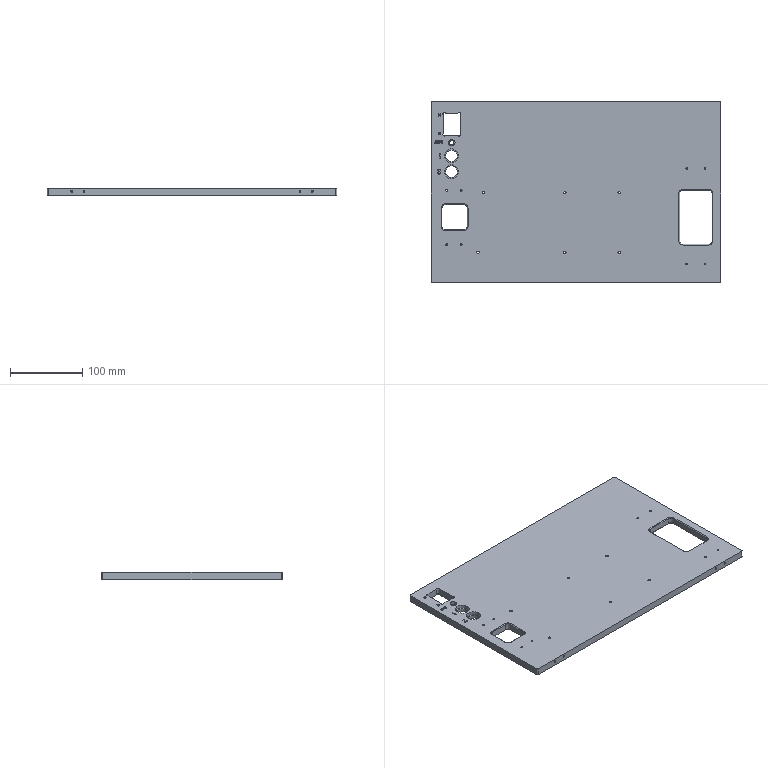CAM job | NX | 3-axis milling | part box 400 x 250 x 10 mm | stock box 406 x 256 x 10 mm
Tools:
number,name,description,diameter,corner_radius,flute_length,length,flutes
2,D4A45,Milling Tool-5 Parameters,4.0,0.0,2.0,2.0,2
6,D6,Milling Tool-5 Parameters,6.0,0.0,50.0,75.0,2
15,D1.5,Milling Tool-5 Parameters,1.5,0.0,50.0,75.0,2
4,D4,Milling Tool-5 Parameters,4.0,0.0,50.0,75.0,2
Operations:
program,operation,operation_type,tool,method,geometry_group,spindle_rpm,surface_speed,feed_per_tooth,feed_cut,feed_plunge,cut_length_mm,path_length_mm,cut_time_min,machine_time_min
1吸,ZLEVEL_PROFILE_1_COPY_1_COPY_COPY,ZLevelMilling,D4A45,METHOD,A,9500.0,179.0,0.0526,1000.0,100.0,2020.382,6903.499,2.02,2.509
1吸,ZLEVEL_PROFILE_COPY_COPY_1_COPY,ZLevelMilling,D6,METHOD,A,9500.0,179.0,0.1158,2200.0,1000.0,26405.347,26472.047,12.023,12.03
1吸,HOLE_MILLING,CylinderMilling,D6,METHOD,A,9500.0,179.0,0.0789,1500.0,100.0,2635.424,2890.931,1.757,1.782
1吸,ZLEVEL_PROFILE_COPY_COPY_1_COPY_COPY,ZLevelMilling,D4,METHOD,A,9500.0,179.0,0.1158,2200.0,1000.0,8830.707,9482.931,4.076,4.141
1吸,HOLE_MILLING_COPY_1,CylinderMilling,D4,METHOD,A,9500.0,179.0,0.0789,1500.0,100.0,2317.402,2601.509,1.545,1.573
1吸,HOLE_MILLING_COPY,CylinderMilling,D1.5,METHOD,A,9500.0,44.0,0.0526,1000.0,100.0,5142.587,7109.899,5.143,5.339
1吸,ZLEVEL_PROFILE_COPY_COPY_COPY_COPY,ZLevelMilling,D4,MILL_FINISH,A,9500.0,119.0,0.0632,1200.0,1000.0,1314.261,1390.961,1.096,1.103
1吸,ZLEVEL_PROFILE_COPY_COPY_COPY_COPY_COPY,ZLevelMilling,D4,MILL_FINISH,A,9500.0,119.0,0.0632,1200.0,1000.0,450.873,1181.136,0.3768,0.4498